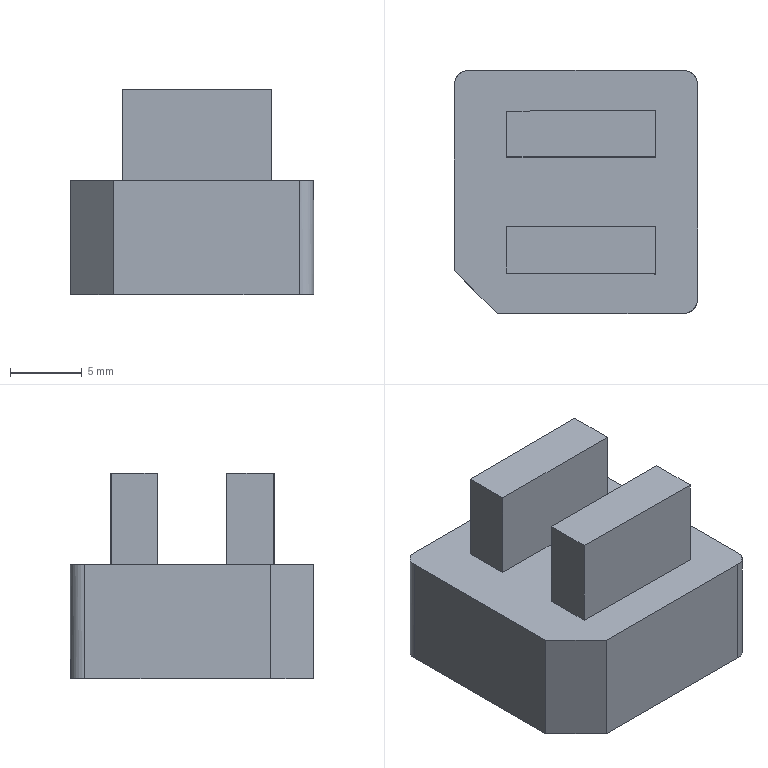NC program | PowerMill | posted with a generic post | part box 17 x 17 x 14.396 mm
Lines 6982 to 7769 of 42940:
N7079 M6
N7080 S18000 M03
N7081 G00 G90 X0.0 Y0.0
N7082 G43 Z10.796 H10
N7083
N7084 G05 P10000 R8
N7085 X6.4224 Y-7.3761
N7086 Z0.7743
N7087 G01 Z-0.4257 F1200.0
N7088 X6.4069 Y-7.3169 F2000.0
N7089 X6.3841 Y-7.2603
N7090 X6.3543 Y-7.207
N7091 X6.3178 Y-7.1577
N7092 X6.2751 Y-7.1134
N7093 X6.2268 Y-7.0746
N7094 X6.1739 Y-7.0424
N7095 X6.1176 Y-7.0173
N7096 X6.0588 Y-6.9998
N7097 X5.9984 Y-6.9899
N7098 X5.9374 Y-6.9878
N7099 X5.8766 Y-6.9934
N7100 X5.8597 Y-6.9964
N7101 X5.7621 Y-7.0153
N7102 X5.6534 Y-7.0287
N7103 X5.5828 Y-7.0339
N7104 X5.512 Y-7.035
N7105 X5.4052 Y-7.0337
N7106 X-3.1195 Y-6.989
N7107 X-4.8763 Y-6.9798
N7108 X-4.9791 Y-6.9753
N7109 X-5.0811 Y-6.9629
N7110 X-5.1816 Y-6.9427
N7111 X-5.2799 Y-6.9147
N7112 X-5.3754 Y-6.8794
N7113 X-5.4674 Y-6.8368
N7114 X-5.5556 Y-6.7873
N7115 X-5.6395 Y-6.731
N7116 X-5.7186 Y-6.6684
N7117 X-5.7933 Y-6.5994
N7118 X-5.8618 Y-6.5251
N7119 X-5.9238 Y-6.4463
N7120 X-5.979 Y-6.3634
N7121 X-6.0207 Y-6.2893
N7122 X-6.0581 Y-6.2122
N7123 X-6.0905 Y-6.1336
N7124 X-6.1179 Y-6.052
N7125 X-6.1401 Y-5.9655
N7126 X-6.1567 Y-5.8712
N7127 X-6.1677 Y-5.7657
N7128 X-6.1729 Y-5.6506
N7129 X-6.1741 Y-5.5393
N7130 X-6.1737 Y-5.4416
N7131 X-6.1706 Y-4.3903
N7132 X-6.1703 Y-3.5568
N7133 X-6.1693 Y-2.7233
N7134 X-6.1676 Y-2.3321
N7135 X-6.1638 Y-2.2699
N7136 X-6.1542 Y-2.2055
N7137 X-6.1376 Y-2.1311
N7138 X-6.1128 Y-2.0458
N7139 X-6.0778 Y-1.9494
N7140 X-6.034 Y-1.8502
N7141 X-5.9889 Y-1.7644
N7142 X-5.9443 Y-1.6925
N7143 X-5.9009 Y-1.6332
N7144 X-5.8558 Y-1.5802
N7145 X-5.7821 Y-1.5036
N7146 X-5.7039 Y-1.4337
N7147 X-5.6218 Y-1.3708
N7148 X-5.5363 Y-1.3152
N7149 X-5.4481 Y-1.2671
N7150 X-5.3577 Y-1.2267
N7151 X-5.2648 Y-1.1938
N7152 X-5.1651 Y-1.167
N7153 X-5.0648 Y-1.1481
N7154 X-4.9642 Y-1.1371
N7155 X-4.8634 Y-1.1341
N7156 X2.7104
N7157 X5.4416
N7158 X5.533 Y-1.135
N7159 X5.6254 Y-1.1389
N7160 X5.7203 Y-1.1474
N7161 X5.8172 Y-1.1629
N7162 X5.9058 Y-1.1842
N7163 X5.9877 Y-1.2106
N7164 X6.0688 Y-1.243
N7165 X6.1591 Y-1.287
N7166 X6.2459 Y-1.3382
N7167 X6.3289 Y-1.3965
N7168 X6.4077 Y-1.4614
N7169 X6.4816 Y-1.5328
N7170 X6.5503 Y-1.6101
N7171 X6.6103 Y-1.6891
N7172 X6.6637 Y-1.7725
N7173 X6.7107 Y-1.8603
N7174 X6.7509 Y-1.9524
N7175 X6.7842 Y-2.0486
N7176 X6.8105 Y-2.1486
N7177 X6.8294 Y-2.2522
N7178 X6.841 Y-2.3591
N7179 X6.8449 Y-2.4691
N7180 X6.8447 Y-2.581
N7181 X6.8435 Y-3.951
N7182 X6.8417 Y-5.0964
N7183 X6.8432 Y-5.7243
N7184 X6.8398 Y-5.8278
N7185 X6.8284 Y-5.9304
N7186 X6.8093 Y-6.0314
N7187 X6.7825 Y-6.13
N7188 X6.7483 Y-6.2257
N7189 X6.7069 Y-6.318
N7190 X6.6586 Y-6.4063
N7191 X6.6035 Y-6.4905
N7192 X6.5422 Y-6.5698
N7193 X6.4731 Y-6.6464
N7194 X6.3987 Y-6.7169
N7195 X6.3196 Y-6.7809
N7196 X6.2365 Y-6.838
N7197 X6.1499 Y-6.888
N7198 X6.0604 Y-6.9305
N7199 X5.9686 Y-6.9655
N7200 X5.8745 Y-6.9928
N7201 X5.8597 Y-6.9964
N7202 X5.778 Y-7.0127 Z-0.4258
N7203 X5.7073 Y-7.0246
N7204 X5.6284 Y-7.0313 Z-0.4259
N7205 X5.5541 Y-7.0352 Z-0.426
N7206 X5.4683 Y-7.0346 Z-0.4261
N7207 X5.3577 Y-7.0334 Z-0.4262
N7208 X-2.0978 Y-6.9944 Z-0.4337
N7209 X-4.8763 Y-6.9798 Z-0.4365
N7210 X-4.9782 Y-6.9754 Z-0.4366
N7211 X-5.0794 Y-6.9632 Z-0.4367
N7212 X-5.1793 Y-6.9431 Z-0.4368
N7213 X-5.2774 Y-6.9154 Z-0.4369
N7214 X-5.3729 Y-6.8801 Z-0.437
N7215 X-5.4654 Y-6.8375 Z-0.4372
N7216 X-5.5543 Y-6.7878 Z-0.4373
N7217 X-5.6387 Y-6.7314 Z-0.4374
N7218 X-5.7182 Y-6.6687 Z-0.4375
N7219 X-5.7925 Y-6.6 Z-0.4376
N7220 X-5.861 Y-6.5259 Z-0.4377
N7221 X-5.9244 Y-6.4456 Z-0.4378
N7222 X-5.981 Y-6.3611 Z-0.4379
N7223 X-6.0306 Y-6.2728 Z-0.438
N7224 X-6.0729 Y-6.1815 Z-0.4381
N7225 X-6.1075 Y-6.0877 Z-0.4382
N7226 X-6.1344 Y-5.9922 Z-0.4383
N7227 X-6.1536 Y-5.8953 Z-0.4384
N7228 X-6.1649 Y-5.7972 Z-0.4385
N7229 X-6.1685 Y-5.6984 Z-0.4386
N7230 X-6.1719 Y-5.2247 Z-0.4391
N7231 X-6.1713 Y-4.5363 Z-0.4397
N7232 X-6.171 Y-3.6966 Z-0.4406
N7233 X-6.1712 Y-3.0558 Z-0.4412
N7234 X-6.1723 Y-2.8956 Z-0.4414
N7235 X-6.1742 Y-2.6859 Z-0.4416
N7236 X-6.1737 Y-2.5257 Z-0.4418
N7237 X-6.1693 Y-2.3655 Z-0.4419
N7238 X-6.1642 Y-2.2903 Z-0.442
N7239 X-6.1534 Y-2.2156 Z-0.4421
N7240 X-6.1353 Y-2.1294 Z-0.4422
N7241 X-6.1082 Y-2.032 Z-0.4423
N7242 X-6.0813 Y-1.9552 Z-0.4424
N7243 X-6.0517 Y-1.8858
N7244 X-6.0056 Y-1.7955 Z-0.4425
N7245 X-5.9533 Y-1.7099 Z-0.4426
N7246 X-5.8947 Y-1.629 Z-0.4428
N7247 X-5.8295 Y-1.5526 Z-0.4429
N7248 X-5.7576 Y-1.4806 Z-0.443
N7249 X-5.6811 Y-1.4147 Z-0.4431
N7250 X-5.5993 Y-1.3548 Z-0.4432
N7251 X-5.5131 Y-1.3015 Z-0.4433
N7252 X-5.4229 Y-1.2551 Z-0.4434
N7253 X-5.3293 Y-1.2159 Z-0.4435
N7254 X-5.2327 Y-1.1841 Z-0.4436
N7255 X-5.134 Y-1.16 Z-0.4437
N7256 X-5.0337 Y-1.1437 Z-0.4438
N7257 X-4.9326 Y-1.1353 Z-0.4439
N7258 X-4.8311 Y-1.1341 Z-0.444
N7259 X2.7719 Y-1.134 Z-0.4517
N7260 X5.5254 Y-1.1331 Z-0.4544
N7261 X5.6316 Y-1.1369 Z-0.4546
N7262 X5.736 Y-1.1486 Z-0.4547
N7263 X5.838 Y-1.1679 Z-0.4548
N7264 X5.9373 Y-1.1948 Z-0.4549
N7265 X6.0334 Y-1.2289 Z-0.455
N7266 X6.1258 Y-1.2702 Z-0.4551
N7267 X6.2141 Y-1.3183 Z-0.4552
N7268 X6.2981 Y-1.373 Z-0.4553
N7269 X6.3776 Y-1.4342 Z-0.4554
N7270 X6.4526 Y-1.502 Z-0.4555
N7271 X6.5222 Y-1.5756 Z-0.4556
N7272 X6.5861 Y-1.6548 Z-0.4557
N7273 X6.6439 Y-1.7391 Z-0.4558
N7274 X6.6951 Y-1.8279 Z-0.4559
N7275 X6.7375 Y-1.9167 Z-0.456
N7276 X6.773 Y-2.0092 Z-0.4561
N7277 X6.8018 Y-2.1062 Z-0.4562
N7278 X6.8235 Y-2.2072 Z-0.4563
N7279 X6.8378 Y-2.3119 Z-0.4564
N7280 X6.8447 Y-2.4197 Z-0.4565
N7281 Y-2.5299 Z-0.4566
N7282 X6.8427 Y-3.2452 Z-0.4574
N7283 X6.8432 Y-3.9511 Z-0.4581
N7284 Y-5.7243 Z-0.4599
N7285 X6.8392 Y-5.8297 Z-0.46
N7286 X6.8274 Y-5.9335 Z-0.4601
N7287 X6.8078 Y-6.0352 Z-0.4602
N7288 X6.7808 Y-6.1341 Z-0.4603
N7289 X6.7465 Y-6.2297 Z-0.4604
N7290 X6.7052 Y-6.3215 Z-0.4605
N7291 X6.6571 Y-6.4091 Z-0.4606
N7292 X6.6024 Y-6.4924 Z-0.4607
N7293 X6.5412 Y-6.5711 Z-0.4608
N7294 X6.4727 Y-6.6464 Z-0.4609
N7295 X6.3985 Y-6.7162 Z-0.461
N7296 X6.319 Y-6.7799 Z-0.4611
N7297 X6.2347 Y-6.8373 Z-0.4612
N7298 X6.1463 Y-6.8878 Z-0.4613
N7299 X6.0542 Y-6.9313 Z-0.4614
N7300 X5.959 Y-6.9674 Z-0.4615
N7301 X5.8613 Y-6.996 Z-0.4616
N7302 X5.8597 Y-6.9964
N7303 X5.778 Y-7.0127 Z-0.4617
N7304 X5.7073 Y-7.0246 Z-0.4618
N7305 X5.6284 Y-7.0313
N7306 X5.5541 Y-7.0352 Z-0.4619
N7307 X5.4683 Y-7.0346 Z-0.462
N7308 X5.3577 Y-7.0334 Z-0.4621
N7309 X-2.0978 Y-6.9944 Z-0.4697
N7310 X-4.8763 Y-6.9798 Z-0.4725
N7311 X-4.9782 Y-6.9754 Z-0.4726
N7312 X-5.0794 Y-6.9632 Z-0.4727
N7313 X-5.1793 Y-6.9431 Z-0.4728
N7314 X-5.2774 Y-6.9154 Z-0.4729
N7315 X-5.3729 Y-6.8801 Z-0.473
N7316 X-5.4654 Y-6.8375 Z-0.4731
N7317 X-5.5543 Y-6.7878 Z-0.4732
N7318 X-5.6387 Y-6.7314 Z-0.4733
N7319 X-5.7182 Y-6.6687 Z-0.4734
N7320 X-5.7925 Y-6.6 Z-0.4735
N7321 X-5.861 Y-6.5259 Z-0.4736
N7322 X-5.9244 Y-6.4456 Z-0.4737
N7323 X-5.981 Y-6.3611 Z-0.4738
N7324 X-6.0306 Y-6.2728 Z-0.4739
N7325 X-6.0729 Y-6.1815 Z-0.474
N7326 X-6.1075 Y-6.0877 Z-0.4741
N7327 X-6.1344 Y-5.9922 Z-0.4742
N7328 X-6.1536 Y-5.8953 Z-0.4743
N7329 X-6.1649 Y-5.7972 Z-0.4744
N7330 X-6.1685 Y-5.6984 Z-0.4745
N7331 X-6.1719 Y-5.2247 Z-0.475
N7332 X-6.1713 Y-4.5363 Z-0.4757
N7333 X-6.171 Y-3.6966 Z-0.4765
N7334 X-6.1712 Y-3.0558 Z-0.4772
N7335 X-6.1723 Y-2.8956 Z-0.4773
N7336 X-6.1742 Y-2.6859 Z-0.4776
N7337 X-6.1737 Y-2.5257 Z-0.4777
N7338 X-6.1693 Y-2.3655 Z-0.4779
N7339 X-6.1642 Y-2.2903 Z-0.478
N7340 X-6.1534 Y-2.2156
N7341 X-6.1353 Y-2.1294 Z-0.4781
N7342 X-6.1082 Y-2.032 Z-0.4782
N7343 X-6.0813 Y-1.9552 Z-0.4783
N7344 X-6.0517 Y-1.8858 Z-0.4784
N7345 X-6.0056 Y-1.7955 Z-0.4785
N7346 X-5.9533 Y-1.7099 Z-0.4786
N7347 X-5.8947 Y-1.629 Z-0.4787
N7348 X-5.8295 Y-1.5526 Z-0.4788
N7349 X-5.7576 Y-1.4806 Z-0.4789
N7350 X-5.6811 Y-1.4147 Z-0.479
N7351 X-5.5993 Y-1.3548 Z-0.4791
N7352 X-5.5131 Y-1.3015 Z-0.4792
N7353 X-5.4229 Y-1.2551 Z-0.4793
N7354 X-5.3293 Y-1.2159 Z-0.4794
N7355 X-5.2327 Y-1.1841 Z-0.4795
N7356 X-5.134 Y-1.16 Z-0.4796
N7357 X-5.0337 Y-1.1437 Z-0.4797
N7358 X-4.9326 Y-1.1353 Z-0.4798
N7359 X-4.8311 Y-1.1341 Z-0.4799
N7360 X2.7719 Y-1.134 Z-0.4876
N7361 X5.5254 Y-1.1331 Z-0.4904
N7362 X5.6316 Y-1.1369 Z-0.4905
N7363 X5.736 Y-1.1486 Z-0.4906
N7364 X5.838 Y-1.1679 Z-0.4907
N7365 X5.9373 Y-1.1948 Z-0.4908
N7366 X6.0334 Y-1.2289 Z-0.4909
N7367 X6.1258 Y-1.2702 Z-0.491
N7368 X6.2141 Y-1.3183 Z-0.4911
N7369 X6.2981 Y-1.373 Z-0.4912
N7370 X6.3776 Y-1.4342 Z-0.4913
N7371 X6.4526 Y-1.502 Z-0.4914
N7372 X6.5222 Y-1.5756 Z-0.4915
N7373 X6.5861 Y-1.6548 Z-0.4916
N7374 X6.6439 Y-1.7391 Z-0.4917
N7375 X6.6951 Y-1.8279 Z-0.4918
N7376 X6.7375 Y-1.9167 Z-0.4919
N7377 X6.773 Y-2.0092 Z-0.492
N7378 X6.8018 Y-2.1062 Z-0.4921
N7379 X6.8235 Y-2.2072 Z-0.4922
N7380 X6.8378 Y-2.3119 Z-0.4923
N7381 X6.8447 Y-2.4197 Z-0.4924
N7382 Y-2.5299 Z-0.4926
N7383 X6.8427 Y-3.2452 Z-0.4933
N7384 X6.8432 Y-3.9511 Z-0.494
N7385 X6.8417 Y-5.0844 Z-0.4951
N7386 X6.8432 Y-5.7243 Z-0.4958
N7387 X6.8398 Y-5.8278 Z-0.4959
N7388 X6.8284 Y-5.9304 Z-0.496
N7389 X6.8093 Y-6.0314 Z-0.4961
N7390 X6.7825 Y-6.13 Z-0.4962
N7391 X6.7483 Y-6.2257 Z-0.4963
N7392 X6.7069 Y-6.318 Z-0.4964
N7393 X6.6586 Y-6.4063 Z-0.4965
N7394 X6.6035 Y-6.4905 Z-0.4966
N7395 X6.5419 Y-6.5701 Z-0.4967
N7396 X6.4736 Y-6.6455 Z-0.4968
N7397 X6.3995 Y-6.7153 Z-0.4969
N7398 X6.3202 Y-6.779 Z-0.497
N7399 X6.2361 Y-6.8365 Z-0.4971
N7400 X6.1477 Y-6.8871 Z-0.4972
N7401 X6.0557 Y-6.9307 Z-0.4973
N7402 X5.9607 Y-6.9669 Z-0.4974
N7403 X5.863 Y-6.9955 Z-0.4975
N7404 X5.8597 Y-6.9964
N7405 X5.778 Y-7.0127 Z-0.4976
N7406 X5.7073 Y-7.0246 Z-0.4977
N7407 X5.6284 Y-7.0313 Z-0.4978
N7408 X5.5541 Y-7.0352 Z-0.4979
N7409 X5.4683 Y-7.0346
N7410 X5.3577 Y-7.0334 Z-0.4981
N7411 X-2.0934 Y-6.9944 Z-0.5056
N7412 X-4.8763 Y-6.9798 Z-0.5084
N7413 X-4.9782 Y-6.9754 Z-0.5085
N7414 X-5.0794 Y-6.9632 Z-0.5086
N7415 X-5.1793 Y-6.9431 Z-0.5087
N7416 X-5.2774 Y-6.9154 Z-0.5088
N7417 X-5.3729 Y-6.8801 Z-0.5089
N7418 X-5.4654 Y-6.8375 Z-0.509
N7419 X-5.5543 Y-6.7878 Z-0.5091
N7420 X-5.6387 Y-6.7314 Z-0.5092
N7421 X-5.7182 Y-6.6687 Z-0.5093
N7422 X-5.7925 Y-6.6001 Z-0.5094
N7423 X-5.861 Y-6.5259 Z-0.5095
N7424 X-5.9244 Y-6.4457 Z-0.5096
N7425 X-5.981 Y-6.3611 Z-0.5097
N7426 X-6.0306 Y-6.2728 Z-0.5098
N7427 X-6.0728 Y-6.1815 Z-0.5099
N7428 X-6.1075 Y-6.0877 Z-0.51
N7429 X-6.1344 Y-5.9922 Z-0.5101
N7430 X-6.1536 Y-5.8953 Z-0.5102
N7431 X-6.1649 Y-5.7972 Z-0.5103
N7432 X-6.1685 Y-5.6984 Z-0.5104
N7433 X-6.172 Y-5.2254 Z-0.5109
N7434 X-6.1713 Y-4.5382 Z-0.5116
N7435 X-6.1711 Y-3.7026 Z-0.5125
N7436 X-6.1712 Y-3.0558 Z-0.5131
N7437 X-6.1723 Y-2.8997 Z-0.5133
N7438 X-6.1743 Y-2.6911 Z-0.5135
N7439 X-6.174 Y-2.535 Z-0.5136
N7440 X-6.17 Y-2.3791 Z-0.5138
N7441 X-6.1653 Y-2.3023 Z-0.5139
N7442 X-6.1553 Y-2.2262
N7443 X-6.1383 Y-2.1418 Z-0.514
N7444 X-6.1112 Y-2.0418 Z-0.5141
N7445 X-6.0838 Y-1.9616 Z-0.5142
N7446 X-6.054 Y-1.8907 Z-0.5143
N7447 X-6.0081 Y-1.8 Z-0.5144
N7448 X-5.9561 Y-1.7141 Z-0.5145
N7449 X-5.8977 Y-1.6329 Z-0.5146
N7450 X-5.8329 Y-1.5562 Z-0.5147
N7451 X-5.7613 Y-1.484 Z-0.5148
N7452 X-5.685 Y-1.4178 Z-0.5149
N7453 X-5.6034 Y-1.3576 Z-0.515
N7454 X-5.5174 Y-1.3039 Z-0.5151
N7455 X-5.4274 Y-1.2572 Z-0.5152
N7456 X-5.334 Y-1.2176 Z-0.5153
N7457 X-5.2375 Y-1.1855 Z-0.5154
N7458 X-5.1388 Y-1.161 Z-0.5155
N7459 X-5.0387 Y-1.1443 Z-0.5156
N7460 X-4.9376 Y-1.1355 Z-0.5157
N7461 X-4.8361 Y-1.1341 Z-0.5158
N7462 X2.3492 Z-0.5231
N7463 X5.5251 Z-0.5263
N7464 X5.6319 Y-1.138 Z-0.5264
N7465 X5.7367 Y-1.1497 Z-0.5265
N7466 X5.8391 Y-1.169 Z-0.5266
N7467 X5.9385 Y-1.1958 Z-0.5267
N7468 X6.0345 Y-1.2298 Z-0.5268
N7469 X6.1267 Y-1.2709 Z-0.5269
N7470 X6.2148 Y-1.3187 Z-0.527
N7471 X6.2984 Y-1.3731 Z-0.5271
N7472 X6.3773 Y-1.4339 Z-0.5272
N7473 X6.4523 Y-1.5016 Z-0.5273
N7474 X6.5219 Y-1.5752 Z-0.5274
N7475 X6.5858 Y-1.6544 Z-0.5276
N7476 X6.6436 Y-1.7387 Z-0.5277
N7477 X6.6949 Y-1.8276 Z-0.5278
N7478 X6.7371 Y-1.9157 Z-0.5279
N7479 X6.7724 Y-2.0077 Z-0.528
N7480 X6.801 Y-2.1043 Z-0.5281
N7481 X6.8228 Y-2.2054 Z-0.5282
N7482 X6.8374 Y-2.3107 Z-0.5283
N7483 X6.8445 Y-2.4197 Z-0.5284
N7484 X6.8449 Y-2.5318 Z-0.5285
N7485 X6.8432 Y-3.7633 Z-0.5297
N7486 X6.8419 Y-4.8967 Z-0.5309
N7487 X6.843 Y-5.6989 Z-0.5317
N7488 X6.8413 Y-5.8026 Z-0.5318
N7489 X6.8319 Y-5.9055 Z-0.5319
N7490 X6.8147 Y-6.0069 Z-0.532
N7491 X6.7898 Y-6.1062 Z-0.5321
N7492 X6.7573 Y-6.2026 Z-0.5322
N7493 X6.7177 Y-6.2958 Z-0.5323
N7494 X6.6711 Y-6.3851 Z-0.5324
N7495 X6.6176 Y-6.4703 Z-0.5325
N7496 X6.5575 Y-6.5511 Z-0.5326
N7497 X6.4906 Y-6.6278 Z-0.5327
N7498 X6.4179 Y-6.6989 Z-0.5328
N7499 X6.3398 Y-6.7642 Z-0.5329
N7500 X6.2568 Y-6.8232 Z-0.533
N7501 X6.1694 Y-6.8755 Z-0.5331
N7502 X6.0783 Y-6.9208 Z-0.5332
N7503 X5.9839 Y-6.9588 Z-0.5333
N7504 X5.8868 Y-6.9893 Z-0.5334
N7505 X5.8597 Y-6.9964 Z-0.5335
N7506 X5.778 Y-7.0127 Z-0.5336
N7507 X5.7073 Y-7.0246
N7508 X5.6284 Y-7.0313 Z-0.5337
N7509 X5.5541 Y-7.0352 Z-0.5338
N7510 X5.4683 Y-7.0346 Z-0.5339
N7511 X5.3577 Y-7.0334 Z-0.534
N7512 X-2.097 Y-6.9944 Z-0.5415
N7513 X-4.8763 Y-6.9798 Z-0.5443
N7514 X-4.9782 Y-6.9754 Z-0.5444
N7515 X-5.0794 Y-6.9632 Z-0.5445
N7516 X-5.1793 Y-6.9431 Z-0.5446
N7517 X-5.2774 Y-6.9154 Z-0.5447
N7518 X-5.3729 Y-6.8801 Z-0.5448
N7519 X-5.4654 Y-6.8375 Z-0.5449
N7520 X-5.5543 Y-6.7878 Z-0.545
N7521 X-5.6387 Y-6.7314 Z-0.5452
N7522 X-5.7182 Y-6.6687 Z-0.5453
N7523 X-5.7925 Y-6.6 Z-0.5454
N7524 X-5.861 Y-6.5259 Z-0.5455
N7525 X-5.9244 Y-6.4457 Z-0.5456
N7526 X-5.981 Y-6.3611 Z-0.5457
N7527 X-6.0306 Y-6.2728 Z-0.5458
N7528 X-6.0729 Y-6.1815 Z-0.5459
N7529 X-6.1075 Y-6.0877 Z-0.546
N7530 X-6.1344 Y-5.9922 Z-0.5461
N7531 X-6.1536 Y-5.8953 Z-0.5462
N7532 X-6.1649 Y-5.7972 Z-0.5463
N7533 X-6.1685 Y-5.6984 Z-0.5464
N7534 X-6.1719 Y-5.2247 Z-0.5468
N7535 X-6.1713 Y-4.5363 Z-0.5475
N7536 X-6.171 Y-3.6966 Z-0.5484
N7537 X-6.1712 Y-3.0558 Z-0.549
N7538 X-6.1723 Y-2.8956 Z-0.5492
N7539 X-6.1742 Y-2.6859 Z-0.5494
N7540 X-6.1737 Y-2.5257 Z-0.5496
N7541 X-6.1693 Y-2.3655 Z-0.5497
N7542 X-6.1642 Y-2.2903 Z-0.5498
N7543 X-6.1534 Y-2.2156 Z-0.5499
N7544 X-6.1353 Y-2.1294 Z-0.55
N7545 X-6.1082 Y-2.032 Z-0.5501
N7546 X-6.0813 Y-1.9552 Z-0.5502
N7547 X-6.0517 Y-1.8858
N7548 X-6.0056 Y-1.7955 Z-0.5503
N7549 X-5.9533 Y-1.7099 Z-0.5504
N7550 X-5.8947 Y-1.629 Z-0.5505
N7551 X-5.8295 Y-1.5526 Z-0.5506
N7552 X-5.7576 Y-1.4806 Z-0.5507
N7553 X-5.6811 Y-1.4147 Z-0.5509
N7554 X-5.5993 Y-1.3548 Z-0.551
N7555 X-5.5131 Y-1.3015 Z-0.5511
N7556 X-5.4229 Y-1.2551 Z-0.5512
N7557 X-5.3293 Y-1.2159 Z-0.5513
N7558 X-5.2327 Y-1.1841 Z-0.5514
N7559 X-5.134 Y-1.16 Z-0.5515
N7560 X-5.0337 Y-1.1437 Z-0.5516
N7561 X-4.9326 Y-1.1353 Z-0.5517
N7562 X-4.8311 Y-1.1341 Z-0.5518
N7563 X2.7718 Y-1.134 Z-0.5595
N7564 X5.5252 Y-1.1331 Z-0.5622
N7565 X5.6315 Y-1.1369 Z-0.5624
N7566 X5.7359 Y-1.1486 Z-0.5625
N7567 X5.838 Y-1.1679 Z-0.5626
N7568 X5.9373 Y-1.1948 Z-0.5627
N7569 X6.0333 Y-1.2289 Z-0.5628
N7570 X6.1257 Y-1.2701 Z-0.5629
N7571 X6.214 Y-1.3182 Z-0.563
N7572 X6.298 Y-1.3729 Z-0.5631
N7573 X6.3775 Y-1.4341 Z-0.5632
N7574 X6.4525 Y-1.5019 Z-0.5633
N7575 X6.5221 Y-1.5755 Z-0.5634
N7576 X6.5861 Y-1.6547 Z-0.5635
N7577 X6.6438 Y-1.739 Z-0.5636
N7578 X6.6951 Y-1.8278 Z-0.5637
N7579 X6.7375 Y-1.9166 Z-0.5638
N7580 X6.773 Y-2.0092 Z-0.5639
N7581 X6.8018 Y-2.1061 Z-0.564
N7582 X6.8235 Y-2.2072 Z-0.5641
N7583 X6.8378 Y-2.3118 Z-0.5642
N7584 X6.8447 Y-2.4196 Z-0.5643
N7585 Y-2.5298 Z-0.5644
N7586 X6.8427 Y-3.2447 Z-0.5651
N7587 X6.8432 Y-3.9511 Z-0.5659
N7588 X6.8417 Y-5.0843 Z-0.567
N7589 X6.8432 Y-5.7243 Z-0.5677
N7590 X6.8398 Y-5.8278 Z-0.5678
N7591 X6.8284 Y-5.9304 Z-0.5679
N7592 X6.8093 Y-6.0314 Z-0.568
N7593 X6.7825 Y-6.13 Z-0.5681
N7594 X6.7483 Y-6.2257 Z-0.5682
N7595 X6.7069 Y-6.318 Z-0.5683
N7596 X6.6586 Y-6.4063 Z-0.5684
N7597 X6.6035 Y-6.4905 Z-0.5685
N7598 X6.5419 Y-6.5701 Z-0.5686
N7599 X6.4736 Y-6.6455 Z-0.5687
N7600 X6.3995 Y-6.7153 Z-0.5688
N7601 X6.3202 Y-6.779 Z-0.5689
N7602 X6.2361 Y-6.8365 Z-0.569
N7603 X6.1477 Y-6.8871 Z-0.5691
N7604 X6.0557 Y-6.9307 Z-0.5692
N7605 X5.9607 Y-6.9669 Z-0.5693
N7606 X5.863 Y-6.9955 Z-0.5694
N7607 X5.8597 Y-6.9964
N7608 X5.778 Y-7.0127 Z-0.5695
N7609 X5.7073 Y-7.0246 Z-0.5696
N7610 X5.6284 Y-7.0313
N7611 X5.5541 Y-7.0352 Z-0.5697
N7612 X5.4683 Y-7.0346 Z-0.5698
N7613 X5.3577 Y-7.0334 Z-0.5699
N7614 X-2.097 Y-6.9944 Z-0.5775
N7615 X-4.8763 Y-6.9798 Z-0.5803
N7616 X-4.9782 Y-6.9754 Z-0.5804
N7617 X-5.0794 Y-6.9632 Z-0.5805
N7618 X-5.1793 Y-6.9431 Z-0.5806
N7619 X-5.2774 Y-6.9154 Z-0.5807
N7620 X-5.3729 Y-6.8801 Z-0.5808
N7621 X-5.4654 Y-6.8375 Z-0.5809
N7622 X-5.5543 Y-6.7878 Z-0.581
N7623 X-5.6387 Y-6.7314 Z-0.5811
N7624 X-5.7182 Y-6.6687 Z-0.5812
N7625 X-5.7925 Y-6.6 Z-0.5813
N7626 X-5.861 Y-6.5259 Z-0.5814
N7627 X-5.9244 Y-6.4457 Z-0.5815
N7628 X-5.981 Y-6.3611 Z-0.5816
N7629 X-6.0306 Y-6.2728 Z-0.5817
N7630 X-6.0729 Y-6.1815 Z-0.5818
N7631 X-6.1075 Y-6.0877 Z-0.5819
N7632 X-6.1344 Y-5.9922 Z-0.582
N7633 X-6.1536 Y-5.8953 Z-0.5821
N7634 X-6.1649 Y-5.7972 Z-0.5822
N7635 X-6.1685 Y-5.6984 Z-0.5823
N7636 X-6.1719 Y-5.2247 Z-0.5828
N7637 X-6.1713 Y-4.5363 Z-0.5835
N7638 X-6.171 Y-3.6966 Z-0.5843
N7639 X-6.1712 Y-3.0558 Z-0.585
N7640 X-6.1723 Y-2.8956 Z-0.5851
N7641 X-6.1742 Y-2.6859 Z-0.5853
N7642 X-6.1737 Y-2.5257 Z-0.5855
N7643 X-6.1693 Y-2.3655 Z-0.5857
N7644 X-6.1642 Y-2.2903
N7645 X-6.1534 Y-2.2156 Z-0.5858
N7646 X-6.1353 Y-2.1294 Z-0.5859
N7647 X-6.1082 Y-2.032 Z-0.586
N7648 X-6.0813 Y-1.9552 Z-0.5861
N7649 X-6.0517 Y-1.8858 Z-0.5862
N7650 X-6.0056 Y-1.7955 Z-0.5863
N7651 X-5.9533 Y-1.7099 Z-0.5864
N7652 X-5.8947 Y-1.629 Z-0.5865
N7653 X-5.8295 Y-1.5526 Z-0.5866
N7654 X-5.7576 Y-1.4806 Z-0.5867
N7655 X-5.6811 Y-1.4147 Z-0.5868
N7656 X-5.5993 Y-1.3548 Z-0.5869
N7657 X-5.5131 Y-1.3015 Z-0.587
N7658 X-5.4229 Y-1.2551 Z-0.5871
N7659 X-5.3293 Y-1.2159 Z-0.5872
N7660 X-5.2327 Y-1.1841 Z-0.5873
N7661 X-5.134 Y-1.16 Z-0.5874
N7662 X-5.0337 Y-1.1437 Z-0.5875
N7663 X-4.9326 Y-1.1353 Z-0.5876
N7664 X-4.8311 Y-1.1341 Z-0.5877
N7665 X2.7718 Y-1.134 Z-0.5954
N7666 X5.5253 Y-1.1331 Z-0.5982
N7667 X5.6315 Y-1.1369 Z-0.5983
N7668 X5.7359 Y-1.1486 Z-0.5984
N7669 X5.838 Y-1.1679 Z-0.5985
N7670 X5.9373 Y-1.1948 Z-0.5986
N7671 X6.0333 Y-1.2289 Z-0.5987
N7672 X6.1257 Y-1.2701 Z-0.5988
N7673 X6.214 Y-1.3182 Z-0.5989
N7674 X6.298 Y-1.3729 Z-0.599
N7675 X6.3775 Y-1.4341 Z-0.5991
N7676 X6.4525 Y-1.5019 Z-0.5992
N7677 X6.5222 Y-1.5755 Z-0.5993
N7678 X6.5861 Y-1.6547 Z-0.5994
N7679 X6.6439 Y-1.739 Z-0.5995
N7680 X6.6951 Y-1.8279 Z-0.5996
N7681 X6.7375 Y-1.9166 Z-0.5997
N7682 X6.773 Y-2.0092 Z-0.5998
N7683 X6.8018 Y-2.1061 Z-0.5999
N7684 X6.8235 Y-2.2072 Z-0.6
N7685 X6.8378 Y-2.3118 Z-0.6001
N7686 X6.8447 Y-2.4196 Z-0.6002
N7687 Y-2.5298 Z-0.6004
N7688 X6.8427 Y-3.2451 Z-0.6011
N7689 X6.8432 Y-3.9511 Z-0.6018
N7690 Y-5.7243 Z-0.6036
N7691 X6.8392 Y-5.8297 Z-0.6037
N7692 X6.8274 Y-5.9335 Z-0.6038
N7693 X6.8078 Y-6.0352 Z-0.6039
N7694 X6.7808 Y-6.1341 Z-0.604
N7695 X6.7465 Y-6.2297 Z-0.6041
N7696 X6.7052 Y-6.3215 Z-0.6042
N7697 X6.6571 Y-6.4091 Z-0.6043
N7698 X6.6024 Y-6.4924 Z-0.6044
N7699 X6.5412 Y-6.5711 Z-0.6045
N7700 X6.4727 Y-6.6464 Z-0.6046
N7701 X6.3985 Y-6.7162 Z-0.6047
N7702 X6.319 Y-6.7799 Z-0.6048
N7703 X6.2347 Y-6.8373 Z-0.6049
N7704 X6.1463 Y-6.8878 Z-0.605
N7705 X6.0542 Y-6.9313 Z-0.6051
N7706 X5.959 Y-6.9674 Z-0.6052
N7707 X5.8613 Y-6.996 Z-0.6053
N7708 X5.8597 Y-6.9964
N7709 X5.778 Y-7.0127 Z-0.6054
N7710 X5.7073 Y-7.0246 Z-0.6055
N7711 X5.6284 Y-7.0313 Z-0.6056
N7712 X5.5541 Y-7.0352
N7713 X5.4683 Y-7.0346 Z-0.6057
N7714 X5.3577 Y-7.0334 Z-0.6058
N7715 X-2.097 Y-6.9944 Z-0.6134
N7716 X-4.8763 Y-6.9798 Z-0.6162
N7717 X-4.9782 Y-6.9754 Z-0.6163
N7718 X-5.0794 Y-6.9632 Z-0.6164
N7719 X-5.1793 Y-6.9431 Z-0.6165
N7720 X-5.2774 Y-6.9154 Z-0.6166
N7721 X-5.3729 Y-6.8801 Z-0.6167
N7722 X-5.4654 Y-6.8375 Z-0.6168
N7723 X-5.5543 Y-6.7878 Z-0.6169
N7724 X-5.6387 Y-6.7314 Z-0.617
N7725 X-5.7182 Y-6.6687 Z-0.6171
N7726 X-5.7925 Y-6.6 Z-0.6172
N7727 X-5.861 Y-6.5259 Z-0.6173
N7728 X-5.9244 Y-6.4457 Z-0.6174
N7729 X-5.981 Y-6.3611 Z-0.6175
N7730 X-6.0306 Y-6.2728 Z-0.6176
N7731 X-6.0729 Y-6.1815 Z-0.6177
N7732 X-6.1075 Y-6.0877 Z-0.6178
N7733 X-6.1344 Y-5.9922 Z-0.6179
N7734 X-6.1536 Y-5.8953 Z-0.618
N7735 X-6.1649 Y-5.7972 Z-0.6181
N7736 X-6.1685 Y-5.6984 Z-0.6182
N7737 X-6.1719 Y-5.2247 Z-0.6187
N7738 X-6.1713 Y-4.5363 Z-0.6194
N7739 X-6.171 Y-3.6966 Z-0.6203
N7740 X-6.1712 Y-3.0558 Z-0.6209
N7741 X-6.1723 Y-2.8956 Z-0.6211
N7742 X-6.1742 Y-2.6859 Z-0.6213
N7743 X-6.1737 Y-2.5257 Z-0.6214
N7744 X-6.1693 Y-2.3655 Z-0.6216
N7745 X-6.1642 Y-2.2903 Z-0.6217
N7746 X-6.1534 Y-2.2156 Z-0.6218
N7747 X-6.1353 Y-2.1294
N7748 X-6.1082 Y-2.032 Z-0.6219
N7749 X-6.0813 Y-1.9552 Z-0.622
N7750 X-6.0517 Y-1.8858 Z-0.6221
N7751 X-6.0056 Y-1.7955 Z-0.6222
N7752 X-5.9533 Y-1.7099 Z-0.6223
N7753 X-5.8947 Y-1.629 Z-0.6224
N7754 X-5.8295 Y-1.5526 Z-0.6225
N7755 X-5.7576 Y-1.4806 Z-0.6226
N7756 X-5.6811 Y-1.4147 Z-0.6227
N7757 X-5.5993 Y-1.3548 Z-0.6228
N7758 X-5.5131 Y-1.3015 Z-0.6229
N7759 X-5.4229 Y-1.2551 Z-0.623
N7760 X-5.3293 Y-1.2159 Z-0.6231
N7761 X-5.2327 Y-1.1841 Z-0.6232
N7762 X-5.134 Y-1.16 Z-0.6233
N7763 X-5.0337 Y-1.1437 Z-0.6234
N7764 X-4.9326 Y-1.1353 Z-0.6235
N7765 X-4.8311 Y-1.1341 Z-0.6236
N7766 X2.7718 Y-1.134 Z-0.6313
N7767 X5.5253 Y-1.1331 Z-0.6341
N7768 X5.6315 Y-1.1369 Z-0.6342
N7769 X5.7359 Y-1.1486 Z-0.6343
N7770 X5.838 Y-1.1679 Z-0.6344
N7771 X5.9373 Y-1.1948 Z-0.6345
N7772 X6.0333 Y-1.2289 Z-0.6346
N7773 X6.1257 Y-1.2701 Z-0.6347
N7774 X6.214 Y-1.3182 Z-0.6348
N7775 X6.298 Y-1.3729 Z-0.6349
N7776 X6.3775 Y-1.4341 Z-0.635
N7777 X6.4525 Y-1.5019 Z-0.6351
N7778 X6.5222 Y-1.5755 Z-0.6352
N7779 X6.5861 Y-1.6547 Z-0.6353
N7780 X6.6439 Y-1.739 Z-0.6354
N7781 X6.6951 Y-1.8279 Z-0.6356
N7782 X6.7375 Y-1.9166 Z-0.6357
N7783 X6.773 Y-2.0092 Z-0.6358
N7784 X6.8018 Y-2.1061 Z-0.6359
N7785 X6.8235 Y-2.2072 Z-0.636
N7786 X6.8378 Y-2.3118 Z-0.6361
N7787 X6.8447 Y-2.4196 Z-0.6362
N7788 Y-2.5298 Z-0.6363
N7789 X6.8427 Y-3.2451 Z-0.637
N7790 X6.8432 Y-3.9511 Z-0.6377
N7791 X6.8417 Y-5.0843 Z-0.6389
N7792 X6.8432 Y-5.7243 Z-0.6395
N7793 X6.8398 Y-5.8278 Z-0.6396
N7794 X6.8284 Y-5.9304 Z-0.6397
N7795 X6.8093 Y-6.0314 Z-0.6398
N7796 X6.7825 Y-6.13 Z-0.6399
N7797 X6.7483 Y-6.2257 Z-0.64
N7798 X6.7069 Y-6.318 Z-0.6401
N7799 X6.6586 Y-6.4063 Z-0.6402
N7800 X6.6035 Y-6.4905 Z-0.6403
N7801 X6.5419 Y-6.5701 Z-0.6404
N7802 X6.4736 Y-6.6455 Z-0.6405
N7803 X6.3995 Y-6.7153 Z-0.6406
N7804 X6.3202 Y-6.779 Z-0.6408
N7805 X6.2361 Y-6.8365 Z-0.6409
N7806 X6.1477 Y-6.8871 Z-0.641
N7807 X6.0557 Y-6.9307 Z-0.6411
N7808 X5.9607 Y-6.9669 Z-0.6412
N7809 X5.863 Y-6.9955 Z-0.6413
N7810 X5.8597 Y-6.9964
N7811 X5.778 Y-7.0127 Z-0.6414
N7812 X5.7073 Y-7.0246
N7813 X5.6284 Y-7.0313 Z-0.6415
N7814 X5.5541 Y-7.0352 Z-0.6416
N7815 X5.4683 Y-7.0346 Z-0.6417
N7816 X5.3577 Y-7.0334 Z-0.6418
N7817 X-2.097 Y-6.9944 Z-0.6493
N7818 X-4.8763 Y-6.9798 Z-0.6521
N7819 X-4.9782 Y-6.9754 Z-0.6522
N7820 X-5.0794 Y-6.9632 Z-0.6523
N7821 X-5.1793 Y-6.9431 Z-0.6524
N7822 X-5.2774 Y-6.9154 Z-0.6525
N7823 X-5.3729 Y-6.8801 Z-0.6526
N7824 X-5.4654 Y-6.8375 Z-0.6527
N7825 X-5.5543 Y-6.7878 Z-0.6528
N7826 X-5.6387 Y-6.7314 Z-0.6529
N7827 X-5.7182 Y-6.6687 Z-0.653
N7828 X-5.7925 Y-6.6 Z-0.6532
N7829 X-5.861 Y-6.5259 Z-0.6533
N7830 X-5.9244 Y-6.4457 Z-0.6534
N7831 X-5.981 Y-6.3611 Z-0.6535
N7832 X-6.0306 Y-6.2728 Z-0.6536
N7833 X-6.0729 Y-6.1815 Z-0.6537
N7834 X-6.1075 Y-6.0877 Z-0.6538
N7835 X-6.1344 Y-5.9922 Z-0.6539
N7836 X-6.1536 Y-5.8953 Z-0.654
N7837 X-6.1649 Y-5.7972 Z-0.6541
N7838 X-6.1685 Y-5.6984 Z-0.6542
N7839 X-6.1719 Y-5.2247 Z-0.6546
N7840 X-6.1713 Y-4.5363 Z-0.6553
N7841 X-6.171 Y-3.6966 Z-0.6562
N7842 X-6.1712 Y-3.0558 Z-0.6568
N7843 X-6.1723 Y-2.8956 Z-0.657
N7844 X-6.1742 Y-2.6859 Z-0.6572
N7845 X-6.1737 Y-2.5257 Z-0.6574
N7846 X-6.1693 Y-2.3655 Z-0.6575
N7847 X-6.1642 Y-2.2903 Z-0.6576
N7848 X-6.1534 Y-2.2156 Z-0.6577
N7849 X-6.1353 Y-2.1294 Z-0.6578
N7850 X-6.1082 Y-2.032 Z-0.6579
N7851 X-6.0813 Y-1.9552 Z-0.658
N7852 X-6.0517 Y-1.8858
N7853 X-6.0056 Y-1.7955 Z-0.6581
N7854 X-5.9533 Y-1.7099 Z-0.6582
N7855 X-5.8947 Y-1.629 Z-0.6583
N7856 X-5.8295 Y-1.5526 Z-0.6584
N7857 X-5.7576 Y-1.4806 Z-0.6585
N7858 X-5.6811 Y-1.4147 Z-0.6586
N7859 X-5.5993 Y-1.3548 Z-0.6587
N7860 X-5.5131 Y-1.3015 Z-0.6589
N7861 X-5.4229 Y-1.2551 Z-0.659
N7862 X-5.3293 Y-1.2159 Z-0.6591
N7863 X-5.2327 Y-1.1841 Z-0.6592
N7864 X-5.134 Y-1.16 Z-0.6593
N7865 X-5.0337 Y-1.1437 Z-0.6594
N7866 X-4.9326 Y-1.1353 Z-0.6595